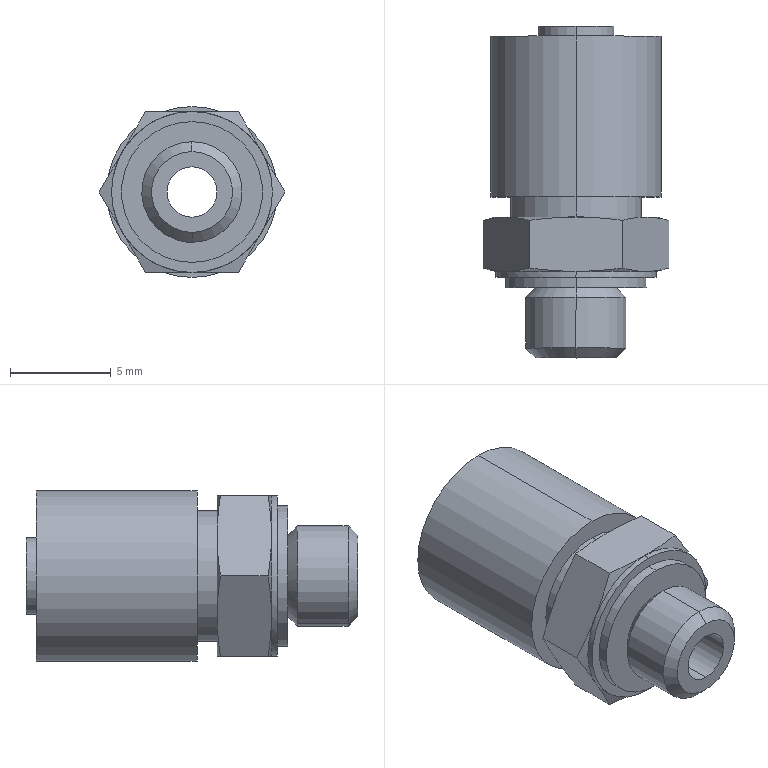Part | SolidWorks | features BaseBody 1 | 1 solid | 43 faces | box 9.238 x 16.5 x 8.5 mm | volume 660.447 mm3 | cone 16 | cylinder 14 | plane 13 | commonest cylinder face diameters 2.5 x2 3.8 x2 5 x2 6.5 x2 7 x2 8 x2
STEP:
#1=CARTESIAN_POINT('',(-3.464,3.5,-2.));
#2=VERTEX_POINT('',#1);
#3=CARTESIAN_POINT('',(-2.309,3.334,-4.));
#4=VERTEX_POINT('',#3);
#5=CARTESIAN_POINT('',(-3.464,3.5,-2.));
#6=CARTESIAN_POINT('',(-3.079,3.5,-2.667));
#7=CARTESIAN_POINT('',(-2.691,3.436,-3.339));
#8=CARTESIAN_POINT('',(-2.309,3.334,-4.));
#9=B_SPLINE_CURVE_WITH_KNOTS('',3,(#5,#6,#7,#8),.UNSPECIFIED.,.F.,.F.,(4,4),(0.,1.),.UNSPECIFIED.);
#10=EDGE_CURVE('',#2,#4,#9,.T.);
#11=ORIENTED_EDGE('',*,*,#10,.F.);
#12=CARTESIAN_POINT('',(0.,3.5,-4.));
#13=VERTEX_POINT('',#12);
#14=CARTESIAN_POINT('',(0.,3.5,0.));
#15=DIRECTION('',(0.,1.,0.));
#16=DIRECTION('',(0.,0.,1.));
#17=AXIS2_PLACEMENT_3D('',#14,#15,#16);
#18=CIRCLE('',#17,4.);
#19=EDGE_CURVE('',#13,#2,#18,.T.);
#20=ORIENTED_EDGE('',*,*,#19,.F.);
#21=CARTESIAN_POINT('',(-2.309,3.334,-4.));
#22=CARTESIAN_POINT('',(-1.546,3.437,-4.));
#23=CARTESIAN_POINT('',(-0.7706,3.5,-4.));
#24=CARTESIAN_POINT('',(0.,3.5,-4.));
#25=B_SPLINE_CURVE_WITH_KNOTS('',3,(#21,#22,#23,#24),.UNSPECIFIED.,.F.,.F.,(4,4),(0.,1.),.UNSPECIFIED.);
#26=EDGE_CURVE('',#4,#13,#25,.T.);
#27=ORIENTED_EDGE('',*,*,#26,.F.);
#28=EDGE_LOOP('',(#11,#20,#27));
#29=FACE_OUTER_BOUND('',#28,.T.);
#30=CARTESIAN_POINT('',(0.,3.5,0.));
#31=DIRECTION('',(0.,-1.,0.));
#32=DIRECTION('',(0.5,0.,0.866));
#33=AXIS2_PLACEMENT_3D('',#30,#31,#32);
#34=CONICAL_SURFACE('',#33,4.,1.309);
#35=ADVANCED_FACE('',(#29),#34,.T.);
#36=ORIENTED_EDGE('',*,*,#26,.T.);
#37=CARTESIAN_POINT('',(2.309,3.334,-4.));
#38=VERTEX_POINT('',#37);
#39=CARTESIAN_POINT('',(0.,3.5,-4.));
#40=CARTESIAN_POINT('',(0.3829,3.5,-4.));
#41=CARTESIAN_POINT('',(0.782,3.484,-4.));
#42=CARTESIAN_POINT('',(1.546,3.427,-4.));
#43=CARTESIAN_POINT('',(1.93,3.385,-4.));
#44=CARTESIAN_POINT('',(2.309,3.334,-4.));
#45=B_SPLINE_CURVE_WITH_KNOTS('',3,(#39,#40,#41,#42,#43,#44),.UNSPECIFIED.,.F.,.F.,(4,2,4),(0.,0.5,1.),.UNSPECIFIED.);
#46=EDGE_CURVE('',#13,#38,#45,.T.);
#47=ORIENTED_EDGE('',*,*,#46,.T.);
#48=CARTESIAN_POINT('',(2.309,0.9658,-4.));
#49=VERTEX_POINT('',#48);
#50=CARTESIAN_POINT('',(2.309,3.5,-4.));
#51=DIRECTION('',(0.,-1.,0.));
#52=VECTOR('',#51,1000.);
#53=LINE('',#50,#52);
#54=EDGE_CURVE('',#38,#49,#53,.T.);
#55=ORIENTED_EDGE('',*,*,#54,.T.);
#56=CARTESIAN_POINT('',(0.,0.8,-4.));
#57=VERTEX_POINT('',#56);
#58=CARTESIAN_POINT('',(2.309,0.9658,-4.));
#59=CARTESIAN_POINT('',(1.546,0.8635,-4.));
#60=CARTESIAN_POINT('',(0.7706,0.8,-4.));
#61=CARTESIAN_POINT('',(0.,0.8,-4.));
#62=B_SPLINE_CURVE_WITH_KNOTS('',3,(#58,#59,#60,#61),.UNSPECIFIED.,.F.,.F.,(4,4),(0.,1.),.UNSPECIFIED.);
#63=EDGE_CURVE('',#49,#57,#62,.T.);
#64=ORIENTED_EDGE('',*,*,#63,.T.);
#65=CARTESIAN_POINT('',(-2.309,0.9658,-4.));
#66=VERTEX_POINT('',#65);
#67=CARTESIAN_POINT('',(0.,0.8,-4.));
#68=CARTESIAN_POINT('',(-0.3829,0.8,-4.));
#69=CARTESIAN_POINT('',(-0.782,0.8159,-4.));
#70=CARTESIAN_POINT('',(-1.546,0.8731,-4.));
#71=CARTESIAN_POINT('',(-1.93,0.915,-4.));
#72=CARTESIAN_POINT('',(-2.309,0.9658,-4.));
#73=B_SPLINE_CURVE_WITH_KNOTS('',3,(#67,#68,#69,#70,#71,#72),.UNSPECIFIED.,.F.,.F.,(4,2,4),(0.,0.5,1.),.UNSPECIFIED.);
#74=EDGE_CURVE('',#57,#66,#73,.T.);
#75=ORIENTED_EDGE('',*,*,#74,.T.);
#76=CARTESIAN_POINT('',(-2.309,3.5,-4.));
#77=DIRECTION('',(0.,-1.,0.));
#78=VECTOR('',#77,1000.);
#79=LINE('',#76,#78);
#80=EDGE_CURVE('',#4,#66,#79,.T.);
#81=ORIENTED_EDGE('',*,*,#80,.F.);
#82=EDGE_LOOP('',(#36,#47,#55,#64,#75,#81));
#83=FACE_OUTER_BOUND('',#82,.T.);
#84=CARTESIAN_POINT('',(2.309,3.5,-4.));
#85=DIRECTION('',(0.,0.,1.));
#86=DIRECTION('',(1.,0.,0.));
#87=AXIS2_PLACEMENT_3D('',#84,#85,#86);
#88=PLANE('',#87);
#89=ADVANCED_FACE('',(#83),#88,.F.);
#90=CARTESIAN_POINT('',(-4.619,3.334,0.));
#91=VERTEX_POINT('',#90);
#92=CARTESIAN_POINT('',(-4.619,3.334,0.));
#93=CARTESIAN_POINT('',(-4.237,3.436,-0.6606));
#94=CARTESIAN_POINT('',(-3.849,3.5,-1.333));
#95=CARTESIAN_POINT('',(-3.464,3.5,-2.));
#96=B_SPLINE_CURVE_WITH_KNOTS('',3,(#92,#93,#94,#95),.UNSPECIFIED.,.F.,.F.,(4,4),(0.,1.),.UNSPECIFIED.);
#97=EDGE_CURVE('',#91,#2,#96,.T.);
#98=ORIENTED_EDGE('',*,*,#97,.T.);
#99=ORIENTED_EDGE('',*,*,#10,.T.);
#100=ORIENTED_EDGE('',*,*,#80,.T.);
#101=CARTESIAN_POINT('',(-3.464,0.8,-2.));
#102=VERTEX_POINT('',#101);
#103=CARTESIAN_POINT('',(-2.309,0.9658,-4.));
#104=CARTESIAN_POINT('',(-2.691,0.8636,-3.339));
#105=CARTESIAN_POINT('',(-3.079,0.8,-2.667));
#106=CARTESIAN_POINT('',(-3.464,0.8,-2.));
#107=B_SPLINE_CURVE_WITH_KNOTS('',3,(#103,#104,#105,#106),.UNSPECIFIED.,.F.,.F.,(4,4),(0.,1.),.UNSPECIFIED.);
#108=EDGE_CURVE('',#66,#102,#107,.T.);
#109=ORIENTED_EDGE('',*,*,#108,.T.);
#110=CARTESIAN_POINT('',(-4.619,0.9658,0.));
#111=VERTEX_POINT('',#110);
#112=CARTESIAN_POINT('',(-3.464,0.8,-2.));
#113=CARTESIAN_POINT('',(-3.849,0.8,-1.333));
#114=CARTESIAN_POINT('',(-4.237,0.8636,-0.6606));
#115=CARTESIAN_POINT('',(-4.619,0.9658,0.));
#116=B_SPLINE_CURVE_WITH_KNOTS('',3,(#112,#113,#114,#115),.UNSPECIFIED.,.F.,.F.,(4,4),(0.,1.),.UNSPECIFIED.);
#117=EDGE_CURVE('',#102,#111,#116,.T.);
#118=ORIENTED_EDGE('',*,*,#117,.T.);
#119=CARTESIAN_POINT('',(-4.619,3.5,0.));
#120=DIRECTION('',(0.,-1.,0.));
#121=VECTOR('',#120,1000.);
#122=LINE('',#119,#121);
#123=EDGE_CURVE('',#91,#111,#122,.T.);
#124=ORIENTED_EDGE('',*,*,#123,.F.);
#125=EDGE_LOOP('',(#98,#99,#100,#109,#118,#124));
#126=FACE_OUTER_BOUND('',#125,.T.);
#127=CARTESIAN_POINT('',(-2.309,3.5,-4.));
#128=DIRECTION('',(0.866,0.,0.5));
#129=DIRECTION('',(0.5,0.,-0.866));
#130=AXIS2_PLACEMENT_3D('',#127,#128,#129);
#131=PLANE('',#130);
#132=ADVANCED_FACE('',(#126),#131,.F.);
#133=CARTESIAN_POINT('',(-2.309,3.334,4.));
#134=VERTEX_POINT('',#133);
#135=CARTESIAN_POINT('',(-3.464,3.5,2.));
#136=VERTEX_POINT('',#135);
#137=CARTESIAN_POINT('',(-2.309,3.334,4.));
#138=CARTESIAN_POINT('',(-2.691,3.436,3.339));
#139=CARTESIAN_POINT('',(-3.079,3.5,2.667));
#140=CARTESIAN_POINT('',(-3.464,3.5,2.));
#141=B_SPLINE_CURVE_WITH_KNOTS('',3,(#137,#138,#139,#140),.UNSPECIFIED.,.F.,.F.,(4,4),(0.,1.),.UNSPECIFIED.);
#142=EDGE_CURVE('',#134,#136,#141,.T.);
#143=ORIENTED_EDGE('',*,*,#142,.T.);
#144=CARTESIAN_POINT('',(-3.464,3.5,2.));
#145=CARTESIAN_POINT('',(-3.849,3.5,1.333));
#146=CARTESIAN_POINT('',(-4.237,3.436,0.6606));
#147=CARTESIAN_POINT('',(-4.619,3.334,0.));
#148=B_SPLINE_CURVE_WITH_KNOTS('',3,(#144,#145,#146,#147),.UNSPECIFIED.,.F.,.F.,(4,4),(0.,1.),.UNSPECIFIED.);
#149=EDGE_CURVE('',#136,#91,#148,.T.);
#150=ORIENTED_EDGE('',*,*,#149,.T.);
#151=ORIENTED_EDGE('',*,*,#123,.T.);
#152=CARTESIAN_POINT('',(-3.464,0.8,2.));
#153=VERTEX_POINT('',#152);
#154=CARTESIAN_POINT('',(-4.619,0.9658,0.));
#155=CARTESIAN_POINT('',(-4.237,0.8636,0.6606));
#156=CARTESIAN_POINT('',(-3.849,0.8,1.333));
#157=CARTESIAN_POINT('',(-3.464,0.8,2.));
#158=B_SPLINE_CURVE_WITH_KNOTS('',3,(#154,#155,#156,#157),.UNSPECIFIED.,.F.,.F.,(4,4),(0.,1.),.UNSPECIFIED.);
#159=EDGE_CURVE('',#111,#153,#158,.T.);
#160=ORIENTED_EDGE('',*,*,#159,.T.);
#161=CARTESIAN_POINT('',(-2.309,0.9658,4.));
#162=VERTEX_POINT('',#161);
#163=CARTESIAN_POINT('',(-3.464,0.8,2.));
#164=CARTESIAN_POINT('',(-3.079,0.8,2.667));
#165=CARTESIAN_POINT('',(-2.691,0.8636,3.339));
#166=CARTESIAN_POINT('',(-2.309,0.9658,4.));
#167=B_SPLINE_CURVE_WITH_KNOTS('',3,(#163,#164,#165,#166),.UNSPECIFIED.,.F.,.F.,(4,4),(0.,1.),.UNSPECIFIED.);
#168=EDGE_CURVE('',#153,#162,#167,.T.);
#169=ORIENTED_EDGE('',*,*,#168,.T.);
#170=CARTESIAN_POINT('',(-2.309,3.5,4.));
#171=DIRECTION('',(0.,-1.,0.));
#172=VECTOR('',#171,1000.);
#173=LINE('',#170,#172);
#174=EDGE_CURVE('',#134,#162,#173,.T.);
#175=ORIENTED_EDGE('',*,*,#174,.F.);
#176=EDGE_LOOP('',(#143,#150,#151,#160,#169,#175));
#177=FACE_OUTER_BOUND('',#176,.T.);
#178=CARTESIAN_POINT('',(-4.619,3.5,0.));
#179=DIRECTION('',(0.866,0.,-0.5));
#180=DIRECTION('',(-0.5,0.,-0.866));
#181=AXIS2_PLACEMENT_3D('',#178,#179,#180);
#182=PLANE('',#181);
#183=ADVANCED_FACE('',(#177),#182,.F.);
#184=CARTESIAN_POINT('',(2.309,3.334,4.));
#185=VERTEX_POINT('',#184);
#186=CARTESIAN_POINT('',(0.,3.5,4.));
#187=VERTEX_POINT('',#186);
#188=CARTESIAN_POINT('',(2.309,3.334,4.));
#189=CARTESIAN_POINT('',(1.546,3.437,4.));
#190=CARTESIAN_POINT('',(0.7706,3.5,4.));
#191=CARTESIAN_POINT('',(0.,3.5,4.));
#192=B_SPLINE_CURVE_WITH_KNOTS('',3,(#188,#189,#190,#191),.UNSPECIFIED.,.F.,.F.,(4,4),(0.,1.),.UNSPECIFIED.);
#193=EDGE_CURVE('',#185,#187,#192,.T.);
#194=ORIENTED_EDGE('',*,*,#193,.T.);
#195=CARTESIAN_POINT('',(0.,3.5,4.));
#196=CARTESIAN_POINT('',(-0.3829,3.5,4.));
#197=CARTESIAN_POINT('',(-0.782,3.484,4.));
#198=CARTESIAN_POINT('',(-1.546,3.427,4.));
#199=CARTESIAN_POINT('',(-1.93,3.385,4.));
#200=CARTESIAN_POINT('',(-2.309,3.334,4.));
#201=B_SPLINE_CURVE_WITH_KNOTS('',3,(#195,#196,#197,#198,#199,#200),.UNSPECIFIED.,.F.,.F.,(4,2,4),(0.,0.5,1.),.UNSPECIFIED.);
#202=EDGE_CURVE('',#187,#134,#201,.T.);
#203=ORIENTED_EDGE('',*,*,#202,.T.);
#204=ORIENTED_EDGE('',*,*,#174,.T.);
#205=CARTESIAN_POINT('',(0.,0.8,4.));
#206=VERTEX_POINT('',#205);
#207=CARTESIAN_POINT('',(-2.309,0.9658,4.));
#208=CARTESIAN_POINT('',(-1.546,0.8635,4.));
#209=CARTESIAN_POINT('',(-0.7706,0.8,4.));
#210=CARTESIAN_POINT('',(0.,0.8,4.));
#211=B_SPLINE_CURVE_WITH_KNOTS('',3,(#207,#208,#209,#210),.UNSPECIFIED.,.F.,.F.,(4,4),(0.,1.),.UNSPECIFIED.);
#212=EDGE_CURVE('',#162,#206,#211,.T.);
#213=ORIENTED_EDGE('',*,*,#212,.T.);
#214=CARTESIAN_POINT('',(2.309,0.9658,4.));
#215=VERTEX_POINT('',#214);
#216=CARTESIAN_POINT('',(0.,0.8,4.));
#217=CARTESIAN_POINT('',(0.3829,0.8,4.));
#218=CARTESIAN_POINT('',(0.782,0.8159,4.));
#219=CARTESIAN_POINT('',(1.546,0.8731,4.));
#220=CARTESIAN_POINT('',(1.93,0.915,4.));
#221=CARTESIAN_POINT('',(2.309,0.9658,4.));
#222=B_SPLINE_CURVE_WITH_KNOTS('',3,(#216,#217,#218,#219,#220,#221),.UNSPECIFIED.,.F.,.F.,(4,2,4),(0.,0.5,1.),.UNSPECIFIED.);
#223=EDGE_CURVE('',#206,#215,#222,.T.);
#224=ORIENTED_EDGE('',*,*,#223,.T.);
#225=CARTESIAN_POINT('',(2.309,3.5,4.));
#226=DIRECTION('',(0.,-1.,0.));
#227=VECTOR('',#226,1000.);
#228=LINE('',#225,#227);
#229=EDGE_CURVE('',#185,#215,#228,.T.);
#230=ORIENTED_EDGE('',*,*,#229,.F.);
#231=EDGE_LOOP('',(#194,#203,#204,#213,#224,#230));
#232=FACE_OUTER_BOUND('',#231,.T.);
#233=CARTESIAN_POINT('',(-2.309,3.5,4.));
#234=DIRECTION('',(0.,0.,-1.));
#235=DIRECTION('',(-1.,0.,0.));
#236=AXIS2_PLACEMENT_3D('',#233,#234,#235);
#237=PLANE('',#236);
#238=ADVANCED_FACE('',(#232),#237,.F.);
#239=CARTESIAN_POINT('',(4.619,3.334,0.));
#240=VERTEX_POINT('',#239);
#241=CARTESIAN_POINT('',(3.464,3.5,2.));
#242=VERTEX_POINT('',#241);
#243=CARTESIAN_POINT('',(4.619,3.334,0.));
#244=CARTESIAN_POINT('',(4.237,3.436,0.6606));
#245=CARTESIAN_POINT('',(3.849,3.5,1.333));
#246=CARTESIAN_POINT('',(3.464,3.5,2.));
#247=B_SPLINE_CURVE_WITH_KNOTS('',3,(#243,#244,#245,#246),.UNSPECIFIED.,.F.,.F.,(4,4),(0.,1.),.UNSPECIFIED.);
#248=EDGE_CURVE('',#240,#242,#247,.T.);
#249=ORIENTED_EDGE('',*,*,#248,.T.);
#250=CARTESIAN_POINT('',(3.464,3.5,2.));
#251=CARTESIAN_POINT('',(3.079,3.5,2.667));
#252=CARTESIAN_POINT('',(2.691,3.436,3.339));
#253=CARTESIAN_POINT('',(2.309,3.334,4.));
#254=B_SPLINE_CURVE_WITH_KNOTS('',3,(#250,#251,#252,#253),.UNSPECIFIED.,.F.,.F.,(4,4),(0.,1.),.UNSPECIFIED.);
#255=EDGE_CURVE('',#242,#185,#254,.T.);
#256=ORIENTED_EDGE('',*,*,#255,.T.);
#257=ORIENTED_EDGE('',*,*,#229,.T.);
#258=CARTESIAN_POINT('',(3.464,0.8,2.));
#259=VERTEX_POINT('',#258);
#260=CARTESIAN_POINT('',(2.309,0.9658,4.));
#261=CARTESIAN_POINT('',(2.691,0.8636,3.339));
#262=CARTESIAN_POINT('',(3.079,0.8,2.667));
#263=CARTESIAN_POINT('',(3.464,0.8,2.));
#264=B_SPLINE_CURVE_WITH_KNOTS('',3,(#260,#261,#262,#263),.UNSPECIFIED.,.F.,.F.,(4,4),(0.,1.),.UNSPECIFIED.);
#265=EDGE_CURVE('',#215,#259,#264,.T.);
#266=ORIENTED_EDGE('',*,*,#265,.T.);
#267=CARTESIAN_POINT('',(4.619,0.9658,0.));
#268=VERTEX_POINT('',#267);
#269=CARTESIAN_POINT('',(3.464,0.8,2.));
#270=CARTESIAN_POINT('',(3.849,0.8,1.333));
#271=CARTESIAN_POINT('',(4.237,0.8636,0.6606));
#272=CARTESIAN_POINT('',(4.619,0.9658,0.));
#273=B_SPLINE_CURVE_WITH_KNOTS('',3,(#269,#270,#271,#272),.UNSPECIFIED.,.F.,.F.,(4,4),(0.,1.),.UNSPECIFIED.);
#274=EDGE_CURVE('',#259,#268,#273,.T.);
#275=ORIENTED_EDGE('',*,*,#274,.T.);
#276=CARTESIAN_POINT('',(4.619,3.5,0.));
#277=DIRECTION('',(0.,-1.,0.));
#278=VECTOR('',#277,1000.);
#279=LINE('',#276,#278);
#280=EDGE_CURVE('',#240,#268,#279,.T.);
#281=ORIENTED_EDGE('',*,*,#280,.F.);
#282=EDGE_LOOP('',(#249,#256,#257,#266,#275,#281));
#283=FACE_OUTER_BOUND('',#282,.T.);
#284=CARTESIAN_POINT('',(2.309,3.5,4.));
#285=DIRECTION('',(-0.866,0.,-0.5));
#286=DIRECTION('',(-0.5,0.,0.866));
#287=AXIS2_PLACEMENT_3D('',#284,#285,#286);
#288=PLANE('',#287);
#289=ADVANCED_FACE('',(#283),#288,.F.);
#290=CARTESIAN_POINT('',(3.464,3.5,-2.));
#291=VERTEX_POINT('',#290);
#292=CARTESIAN_POINT('',(2.309,3.334,-4.));
#293=CARTESIAN_POINT('',(2.691,3.436,-3.339));
#294=CARTESIAN_POINT('',(3.079,3.5,-2.667));
#295=CARTESIAN_POINT('',(3.464,3.5,-2.));
#296=B_SPLINE_CURVE_WITH_KNOTS('',3,(#292,#293,#294,#295),.UNSPECIFIED.,.F.,.F.,(4,4),(0.,1.),.UNSPECIFIED.);
#297=EDGE_CURVE('',#38,#291,#296,.T.);
#298=ORIENTED_EDGE('',*,*,#297,.T.);
#299=CARTESIAN_POINT('',(3.464,3.5,-2.));
#300=CARTESIAN_POINT('',(3.849,3.5,-1.333));
#301=CARTESIAN_POINT('',(4.237,3.436,-0.6606));
#302=CARTESIAN_POINT('',(4.619,3.334,0.));
#303=B_SPLINE_CURVE_WITH_KNOTS('',3,(#299,#300,#301,#302),.UNSPECIFIED.,.F.,.F.,(4,4),(0.,1.),.UNSPECIFIED.);
#304=EDGE_CURVE('',#291,#240,#303,.T.);
#305=ORIENTED_EDGE('',*,*,#304,.T.);
#306=ORIENTED_EDGE('',*,*,#280,.T.);
#307=CARTESIAN_POINT('',(3.464,0.8,-2.));
#308=VERTEX_POINT('',#307);
#309=CARTESIAN_POINT('',(4.619,0.9658,0.));
#310=CARTESIAN_POINT('',(4.237,0.8636,-0.6606));
#311=CARTESIAN_POINT('',(3.849,0.8,-1.333));
#312=CARTESIAN_POINT('',(3.464,0.8,-2.));
#313=B_SPLINE_CURVE_WITH_KNOTS('',3,(#309,#310,#311,#312),.UNSPECIFIED.,.F.,.F.,(4,4),(0.,1.),.UNSPECIFIED.);
#314=EDGE_CURVE('',#268,#308,#313,.T.);
#315=ORIENTED_EDGE('',*,*,#314,.T.);
#316=CARTESIAN_POINT('',(3.464,0.8,-2.));
#317=CARTESIAN_POINT('',(3.079,0.8,-2.667));
#318=CARTESIAN_POINT('',(2.691,0.8636,-3.339));
#319=CARTESIAN_POINT('',(2.309,0.9658,-4.));
#320=B_SPLINE_CURVE_WITH_KNOTS('',3,(#316,#317,#318,#319),.UNSPECIFIED.,.F.,.F.,(4,4),(0.,1.),.UNSPECIFIED.);
#321=EDGE_CURVE('',#308,#49,#320,.T.);
#322=ORIENTED_EDGE('',*,*,#321,.T.);
#323=ORIENTED_EDGE('',*,*,#54,.F.);
#324=EDGE_LOOP('',(#298,#305,#306,#315,#322,#323));
#325=FACE_OUTER_BOUND('',#324,.T.);
#326=CARTESIAN_POINT('',(4.619,3.5,0.));
#327=DIRECTION('',(-0.866,0.,0.5));
#328=DIRECTION('',(0.5,0.,0.866));
#329=AXIS2_PLACEMENT_3D('',#326,#327,#328);
#330=PLANE('',#329);
#331=ADVANCED_FACE('',(#325),#330,.F.);
#332=ORIENTED_EDGE('',*,*,#321,.F.);
#333=CARTESIAN_POINT('',(0.,0.8,0.));
#334=DIRECTION('',(0.,1.,0.));
#335=DIRECTION('',(0.,0.,1.));
#336=AXIS2_PLACEMENT_3D('',#333,#334,#335);
#337=CIRCLE('',#336,4.);
#338=EDGE_CURVE('',#308,#57,#337,.T.);
#339=ORIENTED_EDGE('',*,*,#338,.T.);
#340=ORIENTED_EDGE('',*,*,#63,.F.);
#341=EDGE_LOOP('',(#332,#339,#340));
#342=FACE_OUTER_BOUND('',#341,.T.);
#343=CARTESIAN_POINT('',(0.,1.872,0.));
#344=DIRECTION('',(0.,1.,0.));
#345=DIRECTION('',(-0.5,0.,0.866));
#346=AXIS2_PLACEMENT_3D('',#343,#344,#345);
#347=CONICAL_SURFACE('',#346,8.,1.309);
#348=ADVANCED_FACE('',(#342),#347,.T.);
#349=CARTESIAN_POINT('',(0.,0.5,-4.));
#350=VERTEX_POINT('',#349);
#351=CARTESIAN_POINT('',(0.,0.5,-4.));
#352=DIRECTION('',(0.,1.,0.));
#353=VECTOR('',#352,1000.);
#354=LINE('',#351,#353);
#355=EDGE_CURVE('',#350,#57,#354,.T.);
#356=ORIENTED_EDGE('',*,*,#355,.T.);
#357=ORIENTED_EDGE('',*,*,#338,.F.);
#358=CARTESIAN_POINT('',(0.,0.8,0.));
#359=DIRECTION('',(0.,1.,0.));
#360=DIRECTION('',(0.,0.,1.));
#361=AXIS2_PLACEMENT_3D('',#358,#359,#360);
#362=CIRCLE('',#361,4.);
#363=EDGE_CURVE('',#259,#308,#362,.T.);
#364=ORIENTED_EDGE('',*,*,#363,.F.);
#365=CARTESIAN_POINT('',(0.,0.8,0.));
#366=DIRECTION('',(0.,1.,0.));
#367=DIRECTION('',(0.,0.,1.));
#368=AXIS2_PLACEMENT_3D('',#365,#366,#367);
#369=CIRCLE('',#368,4.);
#370=EDGE_CURVE('',#206,#259,#369,.T.);
#371=ORIENTED_EDGE('',*,*,#370,.F.);
#372=CARTESIAN_POINT('',(0.,0.5,4.));
#373=VERTEX_POINT('',#372);
#374=CARTESIAN_POINT('',(0.,0.5,4.));
#375=DIRECTION('',(0.,1.,0.));
#376=VECTOR('',#375,1000.);
#377=LINE('',#374,#376);
#378=EDGE_CURVE('',#373,#206,#377,.T.);
#379=ORIENTED_EDGE('',*,*,#378,.F.);
#380=CARTESIAN_POINT('',(0.,0.5,0.));
#381=DIRECTION('',(0.,1.,0.));
#382=DIRECTION('',(0.,0.,1.));
#383=AXIS2_PLACEMENT_3D('',#380,#381,#382);
#384=CIRCLE('',#383,4.);
#385=EDGE_CURVE('',#373,#350,#384,.T.);
#386=ORIENTED_EDGE('',*,*,#385,.T.);
#387=EDGE_LOOP('',(#356,#357,#364,#371,#379,#386));
#388=FACE_OUTER_BOUND('',#387,.T.);
#389=CARTESIAN_POINT('',(0.,13.,0.));
#390=DIRECTION('',(0.,1.,0.));
#391=DIRECTION('',(-1.,0.,0.));
#392=AXIS2_PLACEMENT_3D('',#389,#390,#391);
#393=CYLINDRICAL_SURFACE('',#392,4.);
#394=ADVANCED_FACE('',(#388),#393,.T.);
#395=CARTESIAN_POINT('',(0.,0.5,3.5));
#396=VERTEX_POINT('',#395);
#397=CARTESIAN_POINT('',(0.,0.5,-3.5));
#398=VERTEX_POINT('',#397);
#399=CARTESIAN_POINT('',(0.,0.5,0.));
#400=DIRECTION('',(0.,1.,0.));
#401=DIRECTION('',(0.,0.,1.));
#402=AXIS2_PLACEMENT_3D('',#399,#400,#401);
#403=CIRCLE('',#402,3.5);
#404=EDGE_CURVE('',#396,#398,#403,.T.);
#405=ORIENTED_EDGE('',*,*,#404,.T.);
#406=CARTESIAN_POINT('',(0.,0.5,0.));
#407=DIRECTION('',(0.,1.,0.));
#408=DIRECTION('',(0.,0.,1.));
#409=AXIS2_PLACEMENT_3D('',#406,#407,#408);
#410=CIRCLE('',#409,3.5);
#411=EDGE_CURVE('',#398,#396,#410,.T.);
#412=ORIENTED_EDGE('',*,*,#411,.T.);
#413=EDGE_LOOP('',(#405,#412));
#414=FACE_BOUND('',#413,.T.);
#415=CARTESIAN_POINT('',(0.,0.5,0.));
#416=DIRECTION('',(0.,1.,0.));
#417=DIRECTION('',(0.,0.,1.));
#418=AXIS2_PLACEMENT_3D('',#415,#416,#417);
#419=CIRCLE('',#418,4.);
#420=EDGE_CURVE('',#350,#373,#419,.T.);
#421=ORIENTED_EDGE('',*,*,#420,.F.);
#422=ORIENTED_EDGE('',*,*,#385,.F.);
#423=EDGE_LOOP('',(#421,#422));
#424=FACE_OUTER_BOUND('',#423,.T.);
#425=CARTESIAN_POINT('',(-4.,0.5,0.));
#426=DIRECTION('',(0.,-1.,0.));
#427=DIRECTION('',(0.,0.,-1.));
#428=AXIS2_PLACEMENT_3D('',#425,#426,#427);
#429=PLANE('',#428);
#430=ADVANCED_FACE('',(#414,#424),#429,.T.);
#431=ORIENTED_EDGE('',*,*,#355,.F.);
#432=ORIENTED_EDGE('',*,*,#420,.T.);
#433=ORIENTED_EDGE('',*,*,#378,.T.);
#434=CARTESIAN_POINT('',(0.,0.8,0.));
#435=DIRECTION('',(0.,1.,0.));
#436=DIRECTION('',(0.,0.,1.));
#437=AXIS2_PLACEMENT_3D('',#434,#435,#436);
#438=CIRCLE('',#437,4.);
#439=EDGE_CURVE('',#153,#206,#438,.T.);
#440=ORIENTED_EDGE('',*,*,#439,.F.);
#441=CARTESIAN_POINT('',(0.,0.8,0.));
#442=DIRECTION('',(0.,1.,0.));
#443=DIRECTION('',(0.,0.,1.));
#444=AXIS2_PLACEMENT_3D('',#441,#442,#443);
#445=CIRCLE('',#444,4.);
#446=EDGE_CURVE('',#102,#153,#445,.T.);
#447=ORIENTED_EDGE('',*,*,#446,.F.);
#448=CARTESIAN_POINT('',(0.,0.8,0.));
#449=DIRECTION('',(0.,1.,0.));
#450=DIRECTION('',(0.,0.,1.));
#451=AXIS2_PLACEMENT_3D('',#448,#449,#450);
#452=CIRCLE('',#451,4.);
#453=EDGE_CURVE('',#57,#102,#452,.T.);
#454=ORIENTED_EDGE('',*,*,#453,.F.);
#455=EDGE_LOOP('',(#431,#432,#433,#440,#447,#454));
#456=FACE_OUTER_BOUND('',#455,.T.);
#457=CARTESIAN_POINT('',(0.,13.,0.));
#458=DIRECTION('',(0.,1.,0.));
#459=DIRECTION('',(1.,0.,0.));
#460=AXIS2_PLACEMENT_3D('',#457,#458,#459);
#461=CYLINDRICAL_SURFACE('',#460,4.);
#462=ADVANCED_FACE('',(#456),#461,.T.);
#463=ORIENTED_EDGE('',*,*,#74,.F.);
#464=ORIENTED_EDGE('',*,*,#453,.T.);
#465=ORIENTED_EDGE('',*,*,#108,.F.);
#466=EDGE_LOOP('',(#463,#464,#465));
#467=FACE_OUTER_BOUND('',#466,.T.);
#468=CARTESIAN_POINT('',(0.,1.872,0.));
#469=DIRECTION('',(0.,1.,0.));
#470=DIRECTION('',(0.5,0.,0.866));
#471=AXIS2_PLACEMENT_3D('',#468,#469,#470);
#472=CONICAL_SURFACE('',#471,8.,1.309);
#473=ADVANCED_FACE('',(#467),#472,.T.);
#474=ORIENTED_EDGE('',*,*,#159,.F.);
#475=ORIENTED_EDGE('',*,*,#117,.F.);
#476=ORIENTED_EDGE('',*,*,#446,.T.);
#477=EDGE_LOOP('',(#474,#475,#476));
#478=FACE_OUTER_BOUND('',#477,.T.);
#479=CARTESIAN_POINT('',(0.,1.872,0.));
#480=DIRECTION('',(0.,1.,0.));
#481=DIRECTION('',(1.,0.,0.));
#482=AXIS2_PLACEMENT_3D('',#479,#480,#481);
#483=CONICAL_SURFACE('',#482,8.,1.309);
#484=ADVANCED_FACE('',(#478),#483,.T.);
#485=ORIENTED_EDGE('',*,*,#212,.F.);
#486=ORIENTED_EDGE('',*,*,#168,.F.);
#487=ORIENTED_EDGE('',*,*,#439,.T.);
#488=EDGE_LOOP('',(#485,#486,#487));
#489=FACE_OUTER_BOUND('',#488,.T.);
#490=CARTESIAN_POINT('',(0.,1.872,0.));
#491=DIRECTION('',(0.,1.,0.));
#492=DIRECTION('',(0.5,0.,-0.866));
#493=AXIS2_PLACEMENT_3D('',#490,#491,#492);
#494=CONICAL_SURFACE('',#493,8.,1.309);
#495=ADVANCED_FACE('',(#489),#494,.T.);
#496=CARTESIAN_POINT('',(0.,0.,-3.5));
#497=VERTEX_POINT('',#496);
#498=CARTESIAN_POINT('',(0.,0.,-3.5));
#499=DIRECTION('',(0.,1.,0.));
#500=VECTOR('',#499,1000.);
#501=LINE('',#498,#500);
#502=EDGE_CURVE('',#497,#398,#501,.T.);
#503=ORIENTED_EDGE('',*,*,#502,.F.);
#504=CARTESIAN_POINT('',(0.,0.,3.5));
#505=VERTEX_POINT('',#504);
#506=CARTESIAN_POINT('',(0.,0.,0.));
#507=DIRECTION('',(0.,1.,0.));
#508=DIRECTION('',(0.,0.,1.));
#509=AXIS2_PLACEMENT_3D('',#506,#507,#508);
#510=CIRCLE('',#509,3.5);
#511=EDGE_CURVE('',#497,#505,#510,.T.);
#512=ORIENTED_EDGE('',*,*,#511,.T.);
#513=CARTESIAN_POINT('',(0.,0.,3.5));
#514=DIRECTION('',(0.,1.,0.));
#515=VECTOR('',#514,1000.);
#516=LINE('',#513,#515);
#517=EDGE_CURVE('',#505,#396,#516,.T.);
#518=ORIENTED_EDGE('',*,*,#517,.T.);
#519=ORIENTED_EDGE('',*,*,#411,.F.);
#520=EDGE_LOOP('',(#503,#512,#518,#519));
#521=FACE_OUTER_BOUND('',#520,.T.);
#522=CARTESIAN_POINT('',(0.,13.,0.));
#523=DIRECTION('',(0.,1.,0.));
#524=DIRECTION('',(1.,0.,0.));
#525=AXIS2_PLACEMENT_3D('',#522,#523,#524);
#526=CYLINDRICAL_SURFACE('',#525,3.5);
#527=ADVANCED_FACE('',(#521),#526,.T.);
#528=ORIENTED_EDGE('',*,*,#502,.T.);
#529=ORIENTED_EDGE('',*,*,#404,.F.);
#530=ORIENTED_EDGE('',*,*,#517,.F.);
#531=CARTESIAN_POINT('',(0.,0.,0.));
#532=DIRECTION('',(0.,1.,0.));
#533=DIRECTION('',(0.,0.,1.));
#534=AXIS2_PLACEMENT_3D('',#531,#532,#533);
#535=CIRCLE('',#534,3.5);
#536=EDGE_CURVE('',#505,#497,#535,.T.);
#537=ORIENTED_EDGE('',*,*,#536,.T.);
#538=EDGE_LOOP('',(#528,#529,#530,#537));
#539=FACE_OUTER_BOUND('',#538,.T.);
#540=CARTESIAN_POINT('',(0.,13.,0.));
#541=DIRECTION('',(0.,1.,0.));
#542=DIRECTION('',(-1.,0.,0.));
#543=AXIS2_PLACEMENT_3D('',#540,#541,#542);
#544=CYLINDRICAL_SURFACE('',#543,3.5);
#545=ADVANCED_FACE('',(#539),#544,.T.);
#546=CARTESIAN_POINT('',(0.,0.,2.01));
#547=VERTEX_POINT('',#546);
#548=CARTESIAN_POINT('',(0.,0.,-2.009));
#549=VERTEX_POINT('',#548);
#550=CARTESIAN_POINT('',(0.,0.,0.));
#551=DIRECTION('',(0.,1.,0.));
#552=DIRECTION('',(0.,0.,1.));
#553=AXIS2_PLACEMENT_3D('',#550,#551,#552);
#554=CIRCLE('',#553,2.009);
#555=EDGE_CURVE('',#547,#549,#554,.T.);
#556=ORIENTED_EDGE('',*,*,#555,.T.);
#557=CARTESIAN_POINT('',(0.,0.,0.));
#558=DIRECTION('',(0.,1.,0.));
#559=DIRECTION('',(0.,0.,1.));
#560=AXIS2_PLACEMENT_3D('',#557,#558,#559);
#561=CIRCLE('',#560,2.009);
#562=EDGE_CURVE('',#549,#547,#561,.T.);
#563=ORIENTED_EDGE('',*,*,#562,.T.);
#564=EDGE_LOOP('',(#556,#563));
#565=FACE_BOUND('',#564,.T.);
#566=ORIENTED_EDGE('',*,*,#511,.F.);
#567=ORIENTED_EDGE('',*,*,#536,.F.);
#568=EDGE_LOOP('',(#566,#567));
#569=FACE_OUTER_BOUND('',#568,.T.);
#570=CARTESIAN_POINT('',(-3.5,0.,0.));
#571=DIRECTION('',(0.,-1.,0.));
#572=DIRECTION('',(0.,0.,-1.));
#573=AXIS2_PLACEMENT_3D('',#570,#571,#572);
#574=PLANE('',#573);
#575=ADVANCED_FACE('',(#565,#569),#574,.T.);
#576=CARTESIAN_POINT('',(0.,-0.4905,2.5));
#577=VERTEX_POINT('',#576);
#578=CARTESIAN_POINT('',(0.,0.,2.01));
#579=DIRECTION('',(0.,-0.7071,0.7071));
#580=VECTOR('',#579,1000.);
#581=LINE('',#578,#580);
#582=EDGE_CURVE('',#547,#577,#581,.T.);
#583=ORIENTED_EDGE('',*,*,#582,.F.);
#584=ORIENTED_EDGE('',*,*,#562,.F.);
#585=CARTESIAN_POINT('',(0.,-0.4905,-2.5));
#586=VERTEX_POINT('',#585);
#587=CARTESIAN_POINT('',(0.,0.,-2.009));
#588=DIRECTION('',(0.,-0.7071,-0.7071));
#589=VECTOR('',#588,1000.);
#590=LINE('',#587,#589);
#591=EDGE_CURVE('',#549,#586,#590,.T.);
#592=ORIENTED_EDGE('',*,*,#591,.T.);
#593=CARTESIAN_POINT('',(-0.7725,-0.4905,-2.378));
#594=VERTEX_POINT('',#593);
#595=CARTESIAN_POINT('',(0.,-0.4905,0.));
#596=DIRECTION('',(0.,1.,0.));
#597=DIRECTION('',(0.,0.,1.));
#598=AXIS2_PLACEMENT_3D('',#595,#596,#597);
#599=CIRCLE('',#598,2.5);
#600=EDGE_CURVE('',#586,#594,#599,.T.);
#601=ORIENTED_EDGE('',*,*,#600,.T.);
#602=CARTESIAN_POINT('',(0.,-0.4905,0.));
#603=DIRECTION('',(0.,1.,0.));
#604=DIRECTION('',(0.,0.,1.));
#605=AXIS2_PLACEMENT_3D('',#602,#603,#604);
#606=CIRCLE('',#605,2.5);
#607=EDGE_CURVE('',#594,#577,#606,.T.);
#608=ORIENTED_EDGE('',*,*,#607,.T.);
#609=EDGE_LOOP('',(#583,#584,#592,#601,#608));
#610=FACE_OUTER_BOUND('',#609,.T.);
#611=CARTESIAN_POINT('',(0.,0.,0.));
#612=DIRECTION('',(0.,-1.,0.));
#613=DIRECTION('',(1.,0.,0.));
#614=AXIS2_PLACEMENT_3D('',#611,#612,#613);
#615=CONICAL_SURFACE('',#614,2.009,0.7854);
#616=ADVANCED_FACE('',(#610),#615,.T.);
#617=CARTESIAN_POINT('',(-0.7725,-3.009,-2.378));
#618=VERTEX_POINT('',#617);
#619=CARTESIAN_POINT('',(-0.7725,-3.009,-2.378));
#620=DIRECTION('',(0.,1.,0.));
#621=VECTOR('',#620,1000.);
#622=LINE('',#619,#621);
#623=EDGE_CURVE('',#618,#594,#622,.T.);
#624=ORIENTED_EDGE('',*,*,#623,.F.);
#625=CARTESIAN_POINT('',(0.,-3.009,2.5));
#626=VERTEX_POINT('',#625);
#627=CARTESIAN_POINT('',(0.,-3.009,0.));
#628=DIRECTION('',(0.,1.,0.));
#629=DIRECTION('',(0.,0.,1.));
#630=AXIS2_PLACEMENT_3D('',#627,#628,#629);
#631=CIRCLE('',#630,2.5);
#632=EDGE_CURVE('',#618,#626,#631,.T.);
#633=ORIENTED_EDGE('',*,*,#632,.T.);
#634=CARTESIAN_POINT('',(0.,-3.009,2.5));
#635=DIRECTION('',(0.,1.,0.));
#636=VECTOR('',#635,1000.);
#637=LINE('',#634,#636);
#638=EDGE_CURVE('',#626,#577,#637,.T.);
#639=ORIENTED_EDGE('',*,*,#638,.T.);
#640=ORIENTED_EDGE('',*,*,#607,.F.);
#641=EDGE_LOOP('',(#624,#633,#639,#640));
#642=FACE_OUTER_BOUND('',#641,.T.);
#643=CARTESIAN_POINT('',(0.,13.,0.));
#644=DIRECTION('',(0.,1.,0.));
#645=DIRECTION('',(0.9877,0.,-0.1564));
#646=AXIS2_PLACEMENT_3D('',#643,#644,#645);
#647=CYLINDRICAL_SURFACE('',#646,2.5);
#648=ADVANCED_FACE('',(#642),#647,.T.);
#649=ORIENTED_EDGE('',*,*,#623,.T.);
#650=ORIENTED_EDGE('',*,*,#600,.F.);
#651=CARTESIAN_POINT('',(0.,-0.4905,0.));
#652=DIRECTION('',(0.,1.,0.));
#653=DIRECTION('',(0.,0.,1.));
#654=AXIS2_PLACEMENT_3D('',#651,#652,#653);
#655=CIRCLE('',#654,2.5);
#656=EDGE_CURVE('',#577,#586,#655,.T.);
#657=ORIENTED_EDGE('',*,*,#656,.F.);
#658=ORIENTED_EDGE('',*,*,#638,.F.);
#659=CARTESIAN_POINT('',(0.,-3.009,-2.5));
#660=VERTEX_POINT('',#659);
#661=CARTESIAN_POINT('',(0.,-3.009,0.));
#662=DIRECTION('',(0.,1.,0.));
#663=DIRECTION('',(0.,0.,1.));
#664=AXIS2_PLACEMENT_3D('',#661,#662,#663);
#665=CIRCLE('',#664,2.5);
#666=EDGE_CURVE('',#626,#660,#665,.T.);
#667=ORIENTED_EDGE('',*,*,#666,.T.);
#668=CARTESIAN_POINT('',(0.,-3.009,0.));
#669=DIRECTION('',(0.,1.,0.));
#670=DIRECTION('',(0.,0.,1.));
#671=AXIS2_PLACEMENT_3D('',#668,#669,#670);
#672=CIRCLE('',#671,2.5);
#673=EDGE_CURVE('',#660,#618,#672,.T.);
#674=ORIENTED_EDGE('',*,*,#673,.T.);
#675=EDGE_LOOP('',(#649,#650,#657,#658,#667,#674));
#676=FACE_OUTER_BOUND('',#675,.T.);
#677=CARTESIAN_POINT('',(0.,13.,0.));
#678=DIRECTION('',(0.,1.,0.));
#679=DIRECTION('',(-0.9877,0.,0.1564));
#680=AXIS2_PLACEMENT_3D('',#677,#678,#679);
#681=CYLINDRICAL_SURFACE('',#680,2.5);
#682=ADVANCED_FACE('',(#676),#681,.T.);
#683=CARTESIAN_POINT('',(0.,-3.5,-2.009));
#684=VERTEX_POINT('',#683);
#685=CARTESIAN_POINT('',(0.,-3.5,-2.009));
#686=DIRECTION('',(0.,0.7071,-0.7071));
#687=VECTOR('',#686,1000.);
#688=LINE('',#685,#687);
#689=EDGE_CURVE('',#684,#660,#688,.T.);
#690=ORIENTED_EDGE('',*,*,#689,.F.);
#691=CARTESIAN_POINT('',(0.,-3.5,2.009));
#692=VERTEX_POINT('',#691);
#693=CARTESIAN_POINT('',(0.,-3.5,0.));
#694=DIRECTION('',(0.,1.,0.));
#695=DIRECTION('',(0.,0.,1.));
#696=AXIS2_PLACEMENT_3D('',#693,#694,#695);
#697=CIRCLE('',#696,2.009);
#698=EDGE_CURVE('',#684,#692,#697,.T.);
#699=ORIENTED_EDGE('',*,*,#698,.T.);
#700=CARTESIAN_POINT('',(0.,-3.5,2.009));
#701=DIRECTION('',(0.,0.7071,0.7071));
#702=VECTOR('',#701,1000.);
#703=LINE('',#700,#702);
#704=EDGE_CURVE('',#692,#626,#703,.T.);
#705=ORIENTED_EDGE('',*,*,#704,.T.);
#706=ORIENTED_EDGE('',*,*,#632,.F.);
#707=ORIENTED_EDGE('',*,*,#673,.F.);
#708=EDGE_LOOP('',(#690,#699,#705,#706,#707));
#709=FACE_OUTER_BOUND('',#708,.T.);
#710=CARTESIAN_POINT('',(0.,-3.009,0.));
#711=DIRECTION('',(0.,1.,0.));
#712=DIRECTION('',(1.,0.,0.));
#713=AXIS2_PLACEMENT_3D('',#710,#711,#712);
#714=CONICAL_SURFACE('',#713,2.5,0.7854);
#715=ADVANCED_FACE('',(#709),#714,.T.);
#716=ORIENTED_EDGE('',*,*,#689,.T.);
#717=ORIENTED_EDGE('',*,*,#666,.F.);
#718=ORIENTED_EDGE('',*,*,#704,.F.);
#719=CARTESIAN_POINT('',(0.,-3.5,0.));
#720=DIRECTION('',(0.,1.,0.));
#721=DIRECTION('',(0.,0.,1.));
#722=AXIS2_PLACEMENT_3D('',#719,#720,#721);
#723=CIRCLE('',#722,2.009);
#724=EDGE_CURVE('',#692,#684,#723,.T.);
#725=ORIENTED_EDGE('',*,*,#724,.T.);
#726=EDGE_LOOP('',(#716,#717,#718,#725));
#727=FACE_OUTER_BOUND('',#726,.T.);
#728=CARTESIAN_POINT('',(0.,-3.009,0.));
#729=DIRECTION('',(0.,1.,0.));
#730=DIRECTION('',(-1.,0.,0.));
#731=AXIS2_PLACEMENT_3D('',#728,#729,#730);
#732=CONICAL_SURFACE('',#731,2.5,0.7854);
#733=ADVANCED_FACE('',(#727),#732,.T.);
#734=CARTESIAN_POINT('',(0.,-3.5,1.25));
#735=VERTEX_POINT('',#734);
#736=CARTESIAN_POINT('',(0.,-3.5,-1.25));
#737=VERTEX_POINT('',#736);
#738=CARTESIAN_POINT('',(0.,-3.5,0.));
#739=DIRECTION('',(0.,1.,0.));
#740=DIRECTION('',(0.,0.,1.));
#741=AXIS2_PLACEMENT_3D('',#738,#739,#740);
#742=CIRCLE('',#741,1.25);
#743=EDGE_CURVE('',#735,#737,#742,.T.);
#744=ORIENTED_EDGE('',*,*,#743,.T.);
#745=CARTESIAN_POINT('',(0.,-3.5,0.));
#746=DIRECTION('',(0.,1.,0.));
#747=DIRECTION('',(0.,0.,1.));
#748=AXIS2_PLACEMENT_3D('',#745,#746,#747);
#749=CIRCLE('',#748,1.25);
#750=EDGE_CURVE('',#737,#735,#749,.T.);
#751=ORIENTED_EDGE('',*,*,#750,.T.);
#752=EDGE_LOOP('',(#744,#751));
#753=FACE_BOUND('',#752,.T.);
#754=ORIENTED_EDGE('',*,*,#698,.F.);
#755=ORIENTED_EDGE('',*,*,#724,.F.);
#756=EDGE_LOOP('',(#754,#755));
#757=FACE_OUTER_BOUND('',#756,.T.);
#758=CARTESIAN_POINT('',(-2.009,-3.5,0.));
#759=DIRECTION('',(0.,-1.,0.));
#760=DIRECTION('',(0.,0.,-1.));
#761=AXIS2_PLACEMENT_3D('',#758,#759,#760);
#762=PLANE('',#761);
#763=ADVANCED_FACE('',(#753,#757),#762,.T.);
#764=CARTESIAN_POINT('',(0.,13.,-1.25));
#765=VERTEX_POINT('',#764);
#766=CARTESIAN_POINT('',(0.,-3.5,-1.25));
#767=DIRECTION('',(0.,1.,0.));
#768=VECTOR('',#767,1000.);
#769=LINE('',#766,#768);
#770=EDGE_CURVE('',#737,#765,#769,.T.);
#771=ORIENTED_EDGE('',*,*,#770,.T.);
#772=CARTESIAN_POINT('',(0.,13.,1.25));
#773=VERTEX_POINT('',#772);
#774=CARTESIAN_POINT('',(0.,13.,0.));
#775=DIRECTION('',(0.,1.,0.));
#776=DIRECTION('',(0.,0.,1.));
#777=AXIS2_PLACEMENT_3D('',#774,#775,#776);
#778=CIRCLE('',#777,1.25);
#779=EDGE_CURVE('',#765,#773,#778,.T.);
#780=ORIENTED_EDGE('',*,*,#779,.T.);
#781=CARTESIAN_POINT('',(0.,-3.5,1.25));
#782=DIRECTION('',(0.,1.,0.));
#783=VECTOR('',#782,1000.);
#784=LINE('',#781,#783);
#785=EDGE_CURVE('',#735,#773,#784,.T.);
#786=ORIENTED_EDGE('',*,*,#785,.F.);
#787=ORIENTED_EDGE('',*,*,#750,.F.);
#788=EDGE_LOOP('',(#771,#780,#786,#787));
#789=FACE_OUTER_BOUND('',#788,.T.);
#790=CARTESIAN_POINT('',(0.,13.,0.));
#791=DIRECTION('',(0.,1.,0.));
#792=DIRECTION('',(1.,0.,0.));
#793=AXIS2_PLACEMENT_3D('',#790,#791,#792);
#794=CYLINDRICAL_SURFACE('',#793,1.25);
#795=ADVANCED_FACE('',(#789),#794,.F.);
#796=ORIENTED_EDGE('',*,*,#770,.F.);
#797=ORIENTED_EDGE('',*,*,#743,.F.);
#798=ORIENTED_EDGE('',*,*,#785,.T.);
#799=CARTESIAN_POINT('',(0.,13.,0.));
#800=DIRECTION('',(0.,1.,0.));
#801=DIRECTION('',(0.,0.,1.));
#802=AXIS2_PLACEMENT_3D('',#799,#800,#801);
#803=CIRCLE('',#802,1.25);
#804=EDGE_CURVE('',#773,#765,#803,.T.);
#805=ORIENTED_EDGE('',*,*,#804,.T.);
#806=EDGE_LOOP('',(#796,#797,#798,#805));
#807=FACE_OUTER_BOUND('',#806,.T.);
#808=CARTESIAN_POINT('',(0.,13.,0.));
#809=DIRECTION('',(0.,1.,0.));
#810=DIRECTION('',(-1.,0.,0.));
#811=AXIS2_PLACEMENT_3D('',#808,#809,#810);
#812=CYLINDRICAL_SURFACE('',#811,1.25);
#813=ADVANCED_FACE('',(#807),#812,.F.);
#814=CARTESIAN_POINT('',(0.,13.,1.9));
#815=VERTEX_POINT('',#814);
#816=CARTESIAN_POINT('',(0.,13.,-1.9));
#817=VERTEX_POINT('',#816);
#818=CARTESIAN_POINT('',(0.,13.,0.));
#819=DIRECTION('',(0.,1.,0.));
#820=DIRECTION('',(0.,0.,1.));
#821=AXIS2_PLACEMENT_3D('',#818,#819,#820);
#822=CIRCLE('',#821,1.9);
#823=EDGE_CURVE('',#815,#817,#822,.T.);
#824=ORIENTED_EDGE('',*,*,#823,.T.);
#825=CARTESIAN_POINT('',(0.,13.,0.));
#826=DIRECTION('',(0.,1.,0.));
#827=DIRECTION('',(0.,0.,1.));
#828=AXIS2_PLACEMENT_3D('',#825,#826,#827);
#829=CIRCLE('',#828,1.9);
#830=EDGE_CURVE('',#817,#815,#829,.T.);
#831=ORIENTED_EDGE('',*,*,#830,.T.);
#832=EDGE_LOOP('',(#824,#831));
#833=FACE_OUTER_BOUND('',#832,.T.);
#834=ORIENTED_EDGE('',*,*,#779,.F.);
#835=ORIENTED_EDGE('',*,*,#804,.F.);
#836=EDGE_LOOP('',(#834,#835));
#837=FACE_BOUND('',#836,.T.);
#838=CARTESIAN_POINT('',(-1.25,13.,0.));
#839=DIRECTION('',(0.,1.,0.));
#840=DIRECTION('',(0.,0.,1.));
#841=AXIS2_PLACEMENT_3D('',#838,#839,#840);
#842=PLANE('',#841);
#843=ADVANCED_FACE('',(#833,#837),#842,.T.);
#844=CARTESIAN_POINT('',(0.,12.5,-1.9));
#845=VERTEX_POINT('',#844);
#846=CARTESIAN_POINT('',(0.,12.5,-1.9));
#847=DIRECTION('',(0.,1.,0.));
#848=VECTOR('',#847,1000.);
#849=LINE('',#846,#848);
#850=EDGE_CURVE('',#845,#817,#849,.T.);
#851=ORIENTED_EDGE('',*,*,#850,.F.);
#852=CARTESIAN_POINT('',(0.,12.5,1.9));
#853=VERTEX_POINT('',#852);
#854=CARTESIAN_POINT('',(0.,12.5,0.));
#855=DIRECTION('',(0.,1.,0.));
#856=DIRECTION('',(0.,0.,1.));
#857=AXIS2_PLACEMENT_3D('',#854,#855,#856);
#858=CIRCLE('',#857,1.9);
#859=EDGE_CURVE('',#845,#853,#858,.T.);
#860=ORIENTED_EDGE('',*,*,#859,.T.);
#861=CARTESIAN_POINT('',(0.,12.5,1.9));
#862=DIRECTION('',(0.,1.,0.));
#863=VECTOR('',#862,1000.);
#864=LINE('',#861,#863);
#865=EDGE_CURVE('',#853,#815,#864,.T.);
#866=ORIENTED_EDGE('',*,*,#865,.T.);
#867=ORIENTED_EDGE('',*,*,#830,.F.);
#868=EDGE_LOOP('',(#851,#860,#866,#867));
#869=FACE_OUTER_BOUND('',#868,.T.);
#870=CARTESIAN_POINT('',(0.,13.,0.));
#871=DIRECTION('',(0.,1.,0.));
#872=DIRECTION('',(1.,0.,0.));
#873=AXIS2_PLACEMENT_3D('',#870,#871,#872);
#874=CYLINDRICAL_SURFACE('',#873,1.9);
#875=ADVANCED_FACE('',(#869),#874,.T.);
#876=ORIENTED_EDGE('',*,*,#850,.T.);
#877=ORIENTED_EDGE('',*,*,#823,.F.);
#878=ORIENTED_EDGE('',*,*,#865,.F.);
#879=CARTESIAN_POINT('',(0.,12.5,0.));
#880=DIRECTION('',(0.,1.,0.));
#881=DIRECTION('',(0.,0.,1.));
#882=AXIS2_PLACEMENT_3D('',#879,#880,#881);
#883=CIRCLE('',#882,1.9);
#884=EDGE_CURVE('',#853,#845,#883,.T.);
#885=ORIENTED_EDGE('',*,*,#884,.T.);
#886=EDGE_LOOP('',(#876,#877,#878,#885));
#887=FACE_OUTER_BOUND('',#886,.T.);
#888=CARTESIAN_POINT('',(0.,13.,0.));
#889=DIRECTION('',(0.,1.,0.));
#890=DIRECTION('',(-1.,0.,0.));
#891=AXIS2_PLACEMENT_3D('',#888,#889,#890);
#892=CYLINDRICAL_SURFACE('',#891,1.9);
#893=ADVANCED_FACE('',(#887),#892,.T.);
#894=CARTESIAN_POINT('',(0.,12.5,4.25));
#895=VERTEX_POINT('',#894);
#896=CARTESIAN_POINT('',(0.,12.5,-4.25));
#897=VERTEX_POINT('',#896);
#898=CARTESIAN_POINT('',(0.,12.5,0.));
#899=DIRECTION('',(0.,1.,0.));
#900=DIRECTION('',(0.,0.,1.));
#901=AXIS2_PLACEMENT_3D('',#898,#899,#900);
#902=CIRCLE('',#901,4.25);
#903=EDGE_CURVE('',#895,#897,#902,.T.);
#904=ORIENTED_EDGE('',*,*,#903,.T.);
#905=CARTESIAN_POINT('',(0.,12.5,0.));
#906=DIRECTION('',(0.,1.,0.));
#907=DIRECTION('',(0.,0.,1.));
#908=AXIS2_PLACEMENT_3D('',#905,#906,#907);
#909=CIRCLE('',#908,4.25);
#910=EDGE_CURVE('',#897,#895,#909,.T.);
#911=ORIENTED_EDGE('',*,*,#910,.T.);
#912=EDGE_LOOP('',(#904,#911));
#913=FACE_OUTER_BOUND('',#912,.T.);
#914=ORIENTED_EDGE('',*,*,#859,.F.);
#915=ORIENTED_EDGE('',*,*,#884,.F.);
#916=EDGE_LOOP('',(#914,#915));
#917=FACE_BOUND('',#916,.T.);
#918=CARTESIAN_POINT('',(-1.9,12.5,0.));
#919=DIRECTION('',(0.,1.,0.));
#920=DIRECTION('',(0.,0.,1.));
#921=AXIS2_PLACEMENT_3D('',#918,#919,#920);
#922=PLANE('',#921);
#923=ADVANCED_FACE('',(#913,#917),#922,.T.);
#924=CARTESIAN_POINT('',(0.,4.5,-4.25));
#925=VERTEX_POINT('',#924);
#926=CARTESIAN_POINT('',(0.,4.5,-4.25));
#927=DIRECTION('',(0.,1.,0.));
#928=VECTOR('',#927,1000.);
#929=LINE('',#926,#928);
#930=EDGE_CURVE('',#925,#897,#929,.T.);
#931=ORIENTED_EDGE('',*,*,#930,.F.);
#932=CARTESIAN_POINT('',(0.,4.5,4.25));
#933=VERTEX_POINT('',#932);
#934=CARTESIAN_POINT('',(0.,4.5,0.));
#935=DIRECTION('',(0.,1.,0.));
#936=DIRECTION('',(0.,0.,1.));
#937=AXIS2_PLACEMENT_3D('',#934,#935,#936);
#938=CIRCLE('',#937,4.25);
#939=EDGE_CURVE('',#925,#933,#938,.T.);
#940=ORIENTED_EDGE('',*,*,#939,.T.);
#941=CARTESIAN_POINT('',(0.,4.5,4.25));
#942=DIRECTION('',(0.,1.,0.));
#943=VECTOR('',#942,1000.);
#944=LINE('',#941,#943);
#945=EDGE_CURVE('',#933,#895,#944,.T.);
#946=ORIENTED_EDGE('',*,*,#945,.T.);
#947=ORIENTED_EDGE('',*,*,#910,.F.);
#948=EDGE_LOOP('',(#931,#940,#946,#947));
#949=FACE_OUTER_BOUND('',#948,.T.);
#950=CARTESIAN_POINT('',(0.,13.,0.));
#951=DIRECTION('',(0.,1.,0.));
#952=DIRECTION('',(1.,0.,0.));
#953=AXIS2_PLACEMENT_3D('',#950,#951,#952);
#954=CYLINDRICAL_SURFACE('',#953,4.25);
#955=ADVANCED_FACE('',(#949),#954,.T.);
#956=ORIENTED_EDGE('',*,*,#930,.T.);
#957=ORIENTED_EDGE('',*,*,#903,.F.);
#958=ORIENTED_EDGE('',*,*,#945,.F.);
#959=CARTESIAN_POINT('',(0.,4.5,0.));
#960=DIRECTION('',(0.,1.,0.));
#961=DIRECTION('',(0.,0.,1.));
#962=AXIS2_PLACEMENT_3D('',#959,#960,#961);
#963=CIRCLE('',#962,4.25);
#964=EDGE_CURVE('',#933,#925,#963,.T.);
#965=ORIENTED_EDGE('',*,*,#964,.T.);
#966=EDGE_LOOP('',(#956,#957,#958,#965));
#967=FACE_OUTER_BOUND('',#966,.T.);
#968=CARTESIAN_POINT('',(0.,13.,0.));
#969=DIRECTION('',(0.,1.,0.));
#970=DIRECTION('',(-1.,0.,0.));
#971=AXIS2_PLACEMENT_3D('',#968,#969,#970);
#972=CYLINDRICAL_SURFACE('',#971,4.25);
#973=ADVANCED_FACE('',(#967),#972,.T.);
#974=CARTESIAN_POINT('',(0.,4.5,3.25));
#975=VERTEX_POINT('',#974);
#976=CARTESIAN_POINT('',(0.,4.5,-3.25));
#977=VERTEX_POINT('',#976);
#978=CARTESIAN_POINT('',(0.,4.5,0.));
#979=DIRECTION('',(0.,1.,0.));
#980=DIRECTION('',(0.,0.,1.));
#981=AXIS2_PLACEMENT_3D('',#978,#979,#980);
#982=CIRCLE('',#981,3.25);
#983=EDGE_CURVE('',#975,#977,#982,.T.);
#984=ORIENTED_EDGE('',*,*,#983,.T.);
#985=CARTESIAN_POINT('',(0.,4.5,0.));
#986=DIRECTION('',(0.,1.,0.));
#987=DIRECTION('',(0.,0.,1.));
#988=AXIS2_PLACEMENT_3D('',#985,#986,#987);
#989=CIRCLE('',#988,3.25);
#990=EDGE_CURVE('',#977,#975,#989,.T.);
#991=ORIENTED_EDGE('',*,*,#990,.T.);
#992=EDGE_LOOP('',(#984,#991));
#993=FACE_BOUND('',#992,.T.);
#994=ORIENTED_EDGE('',*,*,#939,.F.);
#995=ORIENTED_EDGE('',*,*,#964,.F.);
#996=EDGE_LOOP('',(#994,#995));
#997=FACE_OUTER_BOUND('',#996,.T.);
#998=CARTESIAN_POINT('',(-4.25,4.5,0.));
#999=DIRECTION('',(0.,-1.,0.));
#1000=DIRECTION('',(0.,0.,-1.));
#1001=AXIS2_PLACEMENT_3D('',#998,#999,#1000);
#1002=PLANE('',#1001);
#1003=ADVANCED_FACE('',(#993,#997),#1002,.T.);
#1004=CARTESIAN_POINT('',(0.,3.5,-3.25));
#1005=VERTEX_POINT('',#1004);
#1006=CARTESIAN_POINT('',(0.,3.5,-3.25));
#1007=DIRECTION('',(0.,1.,0.));
#1008=VECTOR('',#1007,1000.);
#1009=LINE('',#1006,#1008);
#1010=EDGE_CURVE('',#1005,#977,#1009,.T.);
#1011=ORIENTED_EDGE('',*,*,#1010,.F.);
#1012=CARTESIAN_POINT('',(0.,3.5,3.25));
#1013=VERTEX_POINT('',#1012);
#1014=CARTESIAN_POINT('',(0.,3.5,0.));
#1015=DIRECTION('',(0.,1.,0.));
#1016=DIRECTION('',(0.,0.,1.));
#1017=AXIS2_PLACEMENT_3D('',#1014,#1015,#1016);
#1018=CIRCLE('',#1017,3.25);
#1019=EDGE_CURVE('',#1005,#1013,#1018,.T.);
#1020=ORIENTED_EDGE('',*,*,#1019,.T.);
#1021=CARTESIAN_POINT('',(0.,3.5,3.25));
#1022=DIRECTION('',(0.,1.,0.));
#1023=VECTOR('',#1022,1000.);
#1024=LINE('',#1021,#1023);
#1025=EDGE_CURVE('',#1013,#975,#1024,.T.);
#1026=ORIENTED_EDGE('',*,*,#1025,.T.);
#1027=ORIENTED_EDGE('',*,*,#990,.F.);
#1028=EDGE_LOOP('',(#1011,#1020,#1026,#1027));
#1029=FACE_OUTER_BOUND('',#1028,.T.);
#1030=CARTESIAN_POINT('',(0.,13.,0.));
#1031=DIRECTION('',(0.,1.,0.));
#1032=DIRECTION('',(1.,0.,0.));
#1033=AXIS2_PLACEMENT_3D('',#1030,#1031,#1032);
#1034=CYLINDRICAL_SURFACE('',#1033,3.25);
#1035=ADVANCED_FACE('',(#1029),#1034,.T.);
#1036=ORIENTED_EDGE('',*,*,#1010,.T.);
#1037=ORIENTED_EDGE('',*,*,#983,.F.);
#1038=ORIENTED_EDGE('',*,*,#1025,.F.);
#1039=CARTESIAN_POINT('',(0.,3.5,0.));
#1040=DIRECTION('',(0.,1.,0.));
#1041=DIRECTION('',(0.,0.,1.));
#1042=AXIS2_PLACEMENT_3D('',#1039,#1040,#1041);
#1043=CIRCLE('',#1042,3.25);
#1044=EDGE_CURVE('',#1013,#1005,#1043,.T.);
#1045=ORIENTED_EDGE('',*,*,#1044,.T.);
#1046=EDGE_LOOP('',(#1036,#1037,#1038,#1045));
#1047=FACE_OUTER_BOUND('',#1046,.T.);
#1048=CARTESIAN_POINT('',(0.,13.,0.));
#1049=DIRECTION('',(0.,1.,0.));
#1050=DIRECTION('',(-1.,0.,0.));
#1051=AXIS2_PLACEMENT_3D('',#1048,#1049,#1050);
#1052=CYLINDRICAL_SURFACE('',#1051,3.25);
#1053=ADVANCED_FACE('',(#1047),#1052,.T.);
#1054=ORIENTED_EDGE('',*,*,#19,.T.);
#1055=CARTESIAN_POINT('',(0.,3.5,0.));
#1056=DIRECTION('',(0.,1.,0.));
#1057=DIRECTION('',(0.,0.,1.));
#1058=AXIS2_PLACEMENT_3D('',#1055,#1056,#1057);
#1059=CIRCLE('',#1058,4.);
#1060=EDGE_CURVE('',#2,#136,#1059,.T.);
#1061=ORIENTED_EDGE('',*,*,#1060,.T.);
#1062=CARTESIAN_POINT('',(0.,3.5,0.));
#1063=DIRECTION('',(0.,1.,0.));
#1064=DIRECTION('',(0.,0.,1.));
#1065=AXIS2_PLACEMENT_3D('',#1062,#1063,#1064);
#1066=CIRCLE('',#1065,4.);
#1067=EDGE_CURVE('',#136,#187,#1066,.T.);
#1068=ORIENTED_EDGE('',*,*,#1067,.T.);
#1069=CARTESIAN_POINT('',(0.,3.5,0.));
#1070=DIRECTION('',(0.,1.,0.));
#1071=DIRECTION('',(0.,0.,1.));
#1072=AXIS2_PLACEMENT_3D('',#1069,#1070,#1071);
#1073=CIRCLE('',#1072,4.);
#1074=EDGE_CURVE('',#187,#242,#1073,.T.);
#1075=ORIENTED_EDGE('',*,*,#1074,.T.);
#1076=CARTESIAN_POINT('',(0.,3.5,0.));
#1077=DIRECTION('',(0.,1.,0.));
#1078=DIRECTION('',(0.,0.,1.));
#1079=AXIS2_PLACEMENT_3D('',#1076,#1077,#1078);
#1080=CIRCLE('',#1079,4.);
#1081=EDGE_CURVE('',#242,#291,#1080,.T.);
#1082=ORIENTED_EDGE('',*,*,#1081,.T.);
#1083=CARTESIAN_POINT('',(0.,3.5,0.));
#1084=DIRECTION('',(0.,1.,0.));
#1085=DIRECTION('',(0.,0.,1.));
#1086=AXIS2_PLACEMENT_3D('',#1083,#1084,#1085);
#1087=CIRCLE('',#1086,4.);
#1088=EDGE_CURVE('',#291,#13,#1087,.T.);
#1089=ORIENTED_EDGE('',*,*,#1088,.T.);
#1090=EDGE_LOOP('',(#1054,#1061,#1068,#1075,#1082,#1089));
#1091=FACE_OUTER_BOUND('',#1090,.T.);
#1092=ORIENTED_EDGE('',*,*,#1019,.F.);
#1093=ORIENTED_EDGE('',*,*,#1044,.F.);
#1094=EDGE_LOOP('',(#1092,#1093));
#1095=FACE_BOUND('',#1094,.T.);
#1096=CARTESIAN_POINT('',(-3.25,3.5,0.));
#1097=DIRECTION('',(0.,1.,0.));
#1098=DIRECTION('',(0.,0.,1.));
#1099=AXIS2_PLACEMENT_3D('',#1096,#1097,#1098);
#1100=PLANE('',#1099);
#1101=ADVANCED_FACE('',(#1091,#1095),#1100,.T.);
#1102=ORIENTED_EDGE('',*,*,#46,.F.);
#1103=ORIENTED_EDGE('',*,*,#1088,.F.);
#1104=ORIENTED_EDGE('',*,*,#297,.F.);
#1105=EDGE_LOOP('',(#1102,#1103,#1104));
#1106=FACE_OUTER_BOUND('',#1105,.T.);
#1107=CARTESIAN_POINT('',(0.,3.5,0.));
#1108=DIRECTION('',(0.,-1.,0.));
#1109=DIRECTION('',(-0.5,0.,0.866));
#1110=AXIS2_PLACEMENT_3D('',#1107,#1108,#1109);
#1111=CONICAL_SURFACE('',#1110,4.,1.309);
#1112=ADVANCED_FACE('',(#1106),#1111,.T.);
#1113=ORIENTED_EDGE('',*,*,#304,.F.);
#1114=ORIENTED_EDGE('',*,*,#1081,.F.);
#1115=ORIENTED_EDGE('',*,*,#248,.F.);
#1116=EDGE_LOOP('',(#1113,#1114,#1115));
#1117=FACE_OUTER_BOUND('',#1116,.T.);
#1118=CARTESIAN_POINT('',(0.,3.5,0.));
#1119=DIRECTION('',(0.,-1.,0.));
#1120=DIRECTION('',(-1.,0.,0.));
#1121=AXIS2_PLACEMENT_3D('',#1118,#1119,#1120);
#1122=CONICAL_SURFACE('',#1121,4.,1.309);
#1123=ADVANCED_FACE('',(#1117),#1122,.T.);
#1124=ORIENTED_EDGE('',*,*,#255,.F.);
#1125=ORIENTED_EDGE('',*,*,#1074,.F.);
#1126=ORIENTED_EDGE('',*,*,#193,.F.);
#1127=EDGE_LOOP('',(#1124,#1125,#1126));
#1128=FACE_OUTER_BOUND('',#1127,.T.);
#1129=CARTESIAN_POINT('',(0.,3.5,0.));
#1130=DIRECTION('',(0.,-1.,0.));
#1131=DIRECTION('',(-0.5,0.,-0.866));
#1132=AXIS2_PLACEMENT_3D('',#1129,#1130,#1131);
#1133=CONICAL_SURFACE('',#1132,4.,1.309);
#1134=ADVANCED_FACE('',(#1128),#1133,.T.);
#1135=ORIENTED_EDGE('',*,*,#202,.F.);
#1136=ORIENTED_EDGE('',*,*,#1067,.F.);
#1137=ORIENTED_EDGE('',*,*,#142,.F.);
#1138=EDGE_LOOP('',(#1135,#1136,#1137));
#1139=FACE_OUTER_BOUND('',#1138,.T.);
#1140=CARTESIAN_POINT('',(0.,3.5,0.));
#1141=DIRECTION('',(0.,-1.,0.));
#1142=DIRECTION('',(0.5,0.,-0.866));
#1143=AXIS2_PLACEMENT_3D('',#1140,#1141,#1142);
#1144=CONICAL_SURFACE('',#1143,4.,1.309);
#1145=ADVANCED_FACE('',(#1139),#1144,.T.);
#1146=ORIENTED_EDGE('',*,*,#149,.F.);
#1147=ORIENTED_EDGE('',*,*,#1060,.F.);
#1148=ORIENTED_EDGE('',*,*,#97,.F.);
#1149=EDGE_LOOP('',(#1146,#1147,#1148));
#1150=FACE_OUTER_BOUND('',#1149,.T.);
#1151=CARTESIAN_POINT('',(0.,3.5,0.));
#1152=DIRECTION('',(0.,-1.,0.));
#1153=DIRECTION('',(1.,0.,0.));
#1154=AXIS2_PLACEMENT_3D('',#1151,#1152,#1153);
#1155=CONICAL_SURFACE('',#1154,4.,1.309);
#1156=ADVANCED_FACE('',(#1150),#1155,.T.);
#1157=ORIENTED_EDGE('',*,*,#582,.T.);
#1158=ORIENTED_EDGE('',*,*,#656,.T.);
#1159=ORIENTED_EDGE('',*,*,#591,.F.);
#1160=ORIENTED_EDGE('',*,*,#555,.F.);
#1161=EDGE_LOOP('',(#1157,#1158,#1159,#1160));
#1162=FACE_OUTER_BOUND('',#1161,.T.);
#1163=CARTESIAN_POINT('',(0.,0.,0.));
#1164=DIRECTION('',(0.,-1.,0.));
#1165=DIRECTION('',(-1.,0.,0.));
#1166=AXIS2_PLACEMENT_3D('',#1163,#1164,#1165);
#1167=CONICAL_SURFACE('',#1166,2.009,0.7854);
#1168=ADVANCED_FACE('',(#1162),#1167,.T.);
#1169=ORIENTED_EDGE('',*,*,#265,.F.);
#1170=ORIENTED_EDGE('',*,*,#223,.F.);
#1171=ORIENTED_EDGE('',*,*,#370,.T.);
#1172=EDGE_LOOP('',(#1169,#1170,#1171));
#1173=FACE_OUTER_BOUND('',#1172,.T.);
#1174=CARTESIAN_POINT('',(0.,1.872,0.));
#1175=DIRECTION('',(0.,1.,0.));
#1176=DIRECTION('',(-0.5,0.,-0.866));
#1177=AXIS2_PLACEMENT_3D('',#1174,#1175,#1176);
#1178=CONICAL_SURFACE('',#1177,8.,1.309);
#1179=ADVANCED_FACE('',(#1173),#1178,.T.);
#1180=ORIENTED_EDGE('',*,*,#314,.F.);
#1181=ORIENTED_EDGE('',*,*,#274,.F.);
#1182=ORIENTED_EDGE('',*,*,#363,.T.);
#1183=EDGE_LOOP('',(#1180,#1181,#1182));
#1184=FACE_OUTER_BOUND('',#1183,.T.);
#1185=CARTESIAN_POINT('',(0.,1.872,0.));
#1186=DIRECTION('',(0.,1.,0.));
#1187=DIRECTION('',(-1.,0.,0.));
#1188=AXIS2_PLACEMENT_3D('',#1185,#1186,#1187);
#1189=CONICAL_SURFACE('',#1188,8.,1.309);
#1190=ADVANCED_FACE('',(#1184),#1189,.T.);
#1191=CLOSED_SHELL('',(#35,#89,#132,#183,#238,#289,#331,#348,#394,#430,#462,#473,#484,#495,#527,#545,#575,#616,#648,#682,#715,#733,#763,#795,#813,#843,#875,#893,#923,#955,#973,#1003,#1035,#1053,#1101,#1112,#1123,#1134,#1145,#1156,#1168,#1179,#1190));
#1192=MANIFOLD_SOLID_BREP('',#1191);
#1193=CARTESIAN_POINT('',(0.,0.,0.));
#1194=DIRECTION('',(0.,0.,1.));
#1195=DIRECTION('',(1.,0.,0.));
#1196=AXIS2_PLACEMENT_3D('',#1193,#1194,#1195);
#1197=(LENGTH_UNIT()NAMED_UNIT(*)SI_UNIT(.MILLI.,.METRE.));
#1198=UNCERTAINTY_MEASURE_WITH_UNIT(LENGTH_MEASURE(0.00001),#1197,'','');
#1199=(NAMED_UNIT(*)PLANE_ANGLE_UNIT()SI_UNIT($,.RADIAN.));
#1200=(NAMED_UNIT(*)SI_UNIT($,.STERADIAN.)SOLID_ANGLE_UNIT());
#1201=(GEOMETRIC_REPRESENTATION_CONTEXT(3)GLOBAL_UNCERTAINTY_ASSIGNED_CONTEXT((#1198))GLOBAL_UNIT_ASSIGNED_CONTEXT((#1197,#1199,#1200))REPRESENTATION_CONTEXT('',''));
#1202=ADVANCED_BREP_SHAPE_REPRESENTATION('',(#1192,#1196),#1201);